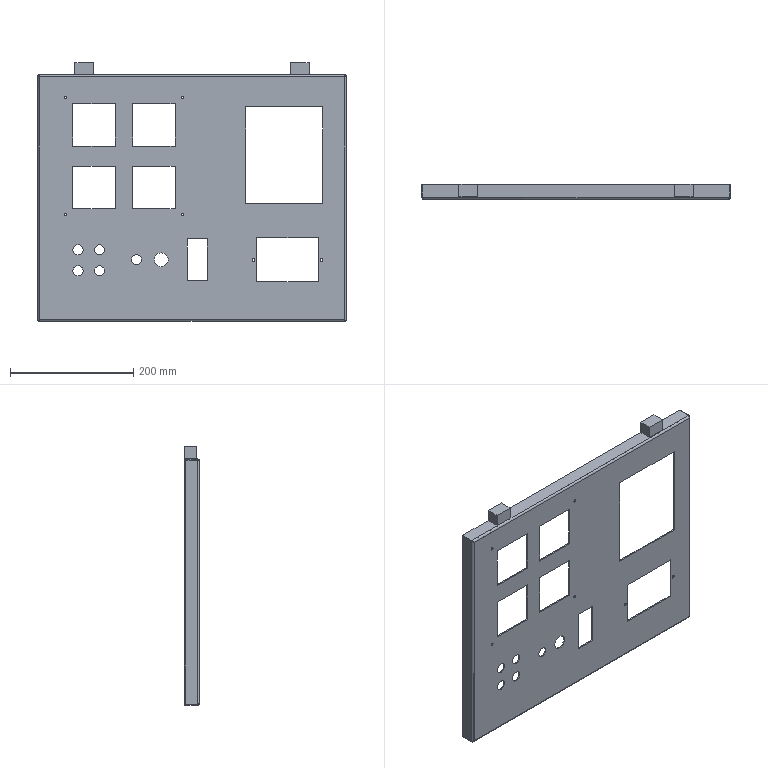Part | STEP file | Station three ctrl box cover | 1 solid | 102 faces | box 500 x 24 x 420 mm | volume 428916 mm3 | plane 60 | cylinder 38 | spline 4 | commonest cylinder face diameters 4.5 x12 16.5 x10 2 x8 6 x4 5 x2 22.5 x2